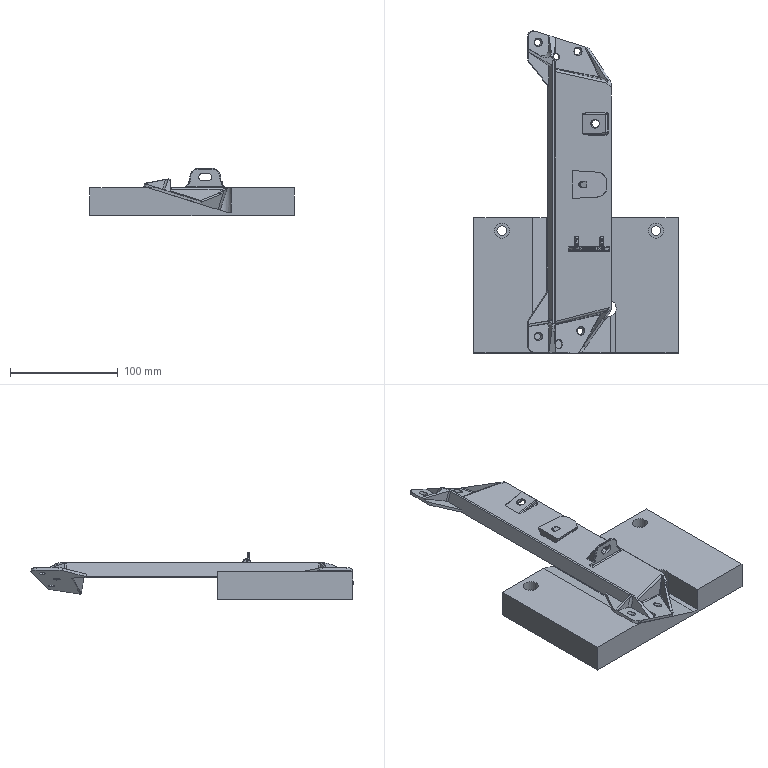NC program | NX | posted with a generic post | part box 190 x 299.709 x 43.804 mm
Lines 1 to 1011 of 6802:
N10 G17 G21 G94 G90
(G-型腔铣-粗 , TOOL : D6-粗刀)
N12 T01 M6
N14 G53
N16 G17 G0 G90 X-26.385 Y-5.888 S5300 M3
N18 G43 Z10. H1
N20 Z0.7
N22 G94 G1 Z-0.3 F2300.
N24 G2 X-29.15 Y-1.613 R3.6
N26 G3 X-28.979 Y0.112 R7.702
N28 G1 Y13.311
N30 G2 X-28.818 Y13.677 R0.5
N32 G3 X-28.659 Y14.001 R0.5
N34 G1 X-28.331 Y17.785
N36 G3 X-28.679 Y18.305 R0.5
N38 G1 X-32.101 Y19.378
N40 X-32.247 Y19.401
N42 X-32.98
N44 G3 X-33.479 Y18.902 R0.5
N46 G1 Y0.073
N48 G2 X-33.737 Y-1.258 R3.202
N50 X-35.553 Y-2.995 R3.2
N52 G3 X-37.656 Y-7.632 R3.6
N54 G1 Z0.7
N56 G0 Z3.
N58 X-26.385 Y-5.888
N60 Z0.401
N62 G1 Z-0.599
N64 G2 X-29.15 Y-1.613 R3.6
N66 G3 X-28.979 Y0.112 R7.702
N68 G1 Y13.311
N70 G2 X-28.818 Y13.677 R0.5
N72 G3 X-28.659 Y14.001 R0.5
N74 G1 X-28.331 Y17.785
N76 G3 X-28.679 Y18.305 R0.5
N78 G1 X-32.101 Y19.378
N80 X-32.247 Y19.401
N82 X-32.98
N84 G3 X-33.479 Y18.902 R0.5
N86 G1 Y0.073
N88 G2 X-33.737 Y-1.258 R3.202
N90 X-35.553 Y-2.995 R3.2
N92 G3 X-37.656 Y-7.632 R3.6
N94 G1 Z0.401
N96 G0 Z3.
N98 X-26.385 Y-5.888
N100 Z0.101
N102 G1 Z-0.899
N104 G2 X-29.15 Y-1.613 R3.6
N106 G3 X-28.979 Y0.112 R7.702
N108 G1 Y13.311
N110 G2 X-28.818 Y13.677 R0.5
N112 G3 X-28.659 Y14.001 R0.5
N114 G1 X-28.331 Y17.785
N116 G3 X-28.679 Y18.305 R0.5
N118 G1 X-32.101 Y19.378
N120 X-32.247 Y19.401
N122 X-32.98
N124 G3 X-33.479 Y18.902 R0.5
N126 G1 Y0.073
N128 G2 X-33.737 Y-1.258 R3.202
N130 X-35.553 Y-2.995 R3.2
N132 G3 X-37.656 Y-7.632 R3.6
N134 G1 Z0.101
N136 G0 Z3.
N138 X-26.385 Y-5.888
N140 Z-0.199
N142 G1 Z-1.199
N144 G2 X-29.15 Y-1.613 R3.6
N146 G3 X-28.979 Y0.112 R7.702
N148 G1 Y13.311
N150 G2 X-28.818 Y13.677 R0.5
N152 G3 X-28.659 Y14.001 R0.5
N154 G1 X-28.331 Y17.785
N156 G3 X-28.679 Y18.305 R0.5
N158 G1 X-32.101 Y19.378
N160 X-32.247 Y19.401
N162 X-32.98
N164 G3 X-33.479 Y18.902 R0.5
N166 G1 Y0.073
N168 G2 X-33.737 Y-1.258 R3.202
N170 X-35.553 Y-2.995 R3.2
N172 G3 X-37.656 Y-7.632 R3.6
N174 G1 Z-0.199
N176 G0 Z3.
N178 X-26.385 Y-5.888
N180 Z-0.498
N182 G1 Z-1.498
N184 G2 X-29.15 Y-1.613 R3.6
N186 G3 X-28.979 Y0.112 R7.702
N188 G1 Y13.312
N190 G2 X-28.818 Y13.677 R0.5
N192 G3 X-28.659 Y14.001 R0.5
N194 G1 X-28.331 Y17.785
N196 G3 X-28.679 Y18.305 R0.5
N198 G1 X-32.102 Y19.378
N200 X-32.246 Y19.401
N202 X-32.98
N204 G3 X-33.479 Y18.902 R0.5
N206 G1 Y0.073
N208 G2 X-33.737 Y-1.258 R3.202
N210 X-35.553 Y-2.995 R3.2
N212 G3 X-37.656 Y-7.632 R3.6
N214 G1 Z-0.498
N216 G0 Z3.
N218 X-26.385 Y-5.888
N220 Z-0.798
N222 G1 Z-1.798
N224 G2 X-29.15 Y-1.613 R3.6
N226 G3 X-28.979 Y0.112 R7.702
N228 G1 Y13.312
N230 G2 X-28.818 Y13.677 R0.5
N232 G3 X-28.659 Y14.001 R0.5
N234 G1 X-28.331 Y17.785
N236 G3 X-28.679 Y18.305 R0.5
N238 G1 X-32.102 Y19.378
N240 X-32.246 Y19.401
N242 X-32.98
N244 G3 X-33.479 Y18.902 R0.5
N246 G1 Y0.073
N248 G2 X-33.737 Y-1.257 R3.202
N250 X-35.553 Y-2.995 R3.2
N252 G3 X-37.656 Y-7.632 R3.6
N254 G1 Z-0.798
N256 G0 Z3.
N258 X-26.385 Y-5.888
N260 Z-1.098
N262 G1 Z-2.098
N264 G2 X-29.15 Y-1.613 R3.6
N266 G3 X-28.979 Y0.112 R7.702
N268 G1 Y13.312
N270 G2 X-28.818 Y13.677 R0.5
N272 G3 X-28.659 Y14.001 R0.5
N274 G1 X-28.331 Y17.785
N276 G3 X-28.679 Y18.305 R0.5
N278 G1 X-32.102 Y19.379
N280 X-32.246 Y19.401
N282 X-32.98
N284 G3 X-33.479 Y18.902 R0.5
N286 G1 Y0.073
N288 G2 X-33.736 Y-1.257 R3.202
N290 X-35.553 Y-2.995 R3.2
N292 G3 X-37.656 Y-7.632 R3.6
N294 G1 Z-1.098
N296 G0 Z3.
N298 X-26.385 Y-5.888
N300 Z-1.397
N302 G1 Z-2.397
N304 G2 X-29.15 Y-1.613 R3.6
N306 G3 X-28.979 Y0.112 R7.702
N308 G1 Y13.312
N310 G2 X-28.818 Y13.677 R0.5
N312 G3 X-28.659 Y14.001 R0.5
N314 G1 X-28.331 Y17.785
N316 G3 X-28.679 Y18.305 R0.5
N318 G1 X-32.102 Y19.379
N320 X-32.246 Y19.401
N322 X-32.98
N324 G3 X-33.479 Y18.902 R0.5
N326 G1 Y0.073
N328 G2 X-33.736 Y-1.257 R3.202
N330 X-35.553 Y-2.995 R3.2
N332 G3 X-37.656 Y-7.632 R3.6
N334 G1 Z-1.397
N336 G0 Z3.
N338 X-26.385 Y-5.888
N340 Z-1.697
N342 G1 Z-2.697
N344 G2 X-29.15 Y-1.613 R3.6
N346 G3 X-28.979 Y0.112 R7.702
N348 G1 Y13.312
N350 G2 X-28.818 Y13.677 R0.5
N352 G3 X-28.659 Y14.001 R0.5
N354 G1 X-28.331 Y17.785
N356 G3 X-28.679 Y18.305 R0.5
N358 G1 X-32.102 Y19.379
N360 X-32.246 Y19.401
N362 X-32.98
N364 G3 X-33.479 Y18.902 R0.5
N366 G1 Y0.073
N368 G2 X-33.736 Y-1.257 R3.202
N370 X-35.553 Y-2.995 R3.2
N372 G3 X-37.656 Y-7.632 R3.6
N374 G1 Z-1.697
N376 G0 Z3.
N378 X-26.385 Y-5.888
N380 Z-1.997
N382 G1 Z-2.997
N384 G2 X-29.15 Y-1.613 R3.6
N386 G3 X-28.979 Y0.112 R7.702
N388 G1 Y13.312
N390 G2 X-28.818 Y13.677 R0.5
N392 G3 X-28.659 Y14.001 R0.5
N394 G1 X-28.331 Y17.785
N396 G3 X-28.679 Y18.305 R0.5
N398 G1 X-32.102 Y19.379
N400 X-32.246 Y19.401
N402 X-32.98
N404 G3 X-33.479 Y18.902 R0.5
N406 G1 Y0.073
N408 G2 X-33.736 Y-1.257 R3.202
N410 X-35.553 Y-2.995 R3.2
N412 G3 X-37.656 Y-7.632 R3.6
N414 G1 Z-1.997
N416 G0 Z3.
N418 X-26.385 Y-5.888
N420 Z-2.296
N422 G1 Z-3.296
N424 G2 X-29.15 Y-1.613 R3.6
N426 G3 X-28.979 Y0.112 R7.702
N428 G1 Y13.313
N430 G2 X-28.818 Y13.677 R0.5
N432 G3 X-28.659 Y14.001 R0.5
N434 G1 X-28.331 Y17.785
N436 G3 X-28.679 Y18.305 R0.5
N438 G1 X-32.102 Y19.379
N440 X-32.246 Y19.401
N442 X-32.98
N444 G3 X-33.479 Y18.902 R0.5
N446 G1 Y0.073
N448 G2 X-33.736 Y-1.257 R3.202
N450 X-35.553 Y-2.995 R3.2
N452 G3 X-37.656 Y-7.632 R3.6
N454 G1 Z-2.296
N456 G0 Z3.
N458 X-26.385 Y-5.888
N460 Z-2.596
N462 G1 Z-3.596
N464 G2 X-29.15 Y-1.613 R3.6
N466 G3 X-28.979 Y0.112 R7.702
N468 G1 Y13.313
N470 G2 X-28.818 Y13.677 R0.5
N472 G3 X-28.659 Y14.001 R0.5
N474 G1 X-28.331 Y17.785
N476 G3 X-28.679 Y18.305 R0.5
N478 G1 X-32.103 Y19.379
N480 X-32.245 Y19.401
N482 X-32.98
N484 G3 X-33.479 Y18.902 R0.5
N486 G1 Y0.073
N488 G2 X-33.736 Y-1.257 R3.202
N490 X-35.553 Y-2.995 R3.2
N492 G3 X-37.656 Y-7.632 R3.6
N494 G1 Z-2.596
N496 G0 Z3.
N498 X-26.385 Y-5.888
N500 Z-2.896
N502 G1 Z-3.896
N504 G2 X-29.15 Y-1.613 R3.6
N506 G3 X-28.979 Y0.112 R7.702
N508 G1 Y13.313
N510 G2 X-28.818 Y13.677 R0.5
N512 G3 X-28.659 Y14.001 R0.5
N514 G1 X-28.331 Y17.785
N516 G3 X-28.679 Y18.305 R0.5
N518 G1 X-32.103 Y19.379
N520 X-32.245 Y19.401
N522 X-32.98
N524 G3 X-33.479 Y18.902 R0.5
N526 G1 Y0.073
N528 G2 X-33.736 Y-1.257 R3.202
N530 X-35.553 Y-2.995 R3.2
N532 G3 X-37.656 Y-7.632 R3.6
N534 G1 Z-2.896
N536 G0 Z3.
N538 X-26.385 Y-5.888
N540 Z-3.195
N542 G1 Z-4.195
N544 G2 X-29.15 Y-1.613 R3.6
N546 G3 X-28.979 Y0.112 R7.702
N548 G1 Y13.313
N550 G2 X-28.818 Y13.677 R0.5
N552 G3 X-28.659 Y14.001 R0.5
N554 G1 X-28.331 Y17.785
N556 G3 X-28.679 Y18.305 R0.5
N558 G1 X-32.103 Y19.379
N560 X-32.245 Y19.401
N562 X-32.98
N564 G3 X-33.479 Y18.902 R0.5
N566 G1 Y0.073
N568 G2 X-33.736 Y-1.256 R3.202
N570 X-35.553 Y-2.995 R3.2
N572 G3 X-37.656 Y-7.632 R3.6
N574 G1 Z-3.195
N576 G0 Z3.
N578 X-26.385 Y-5.888
N580 Z-3.495
N582 G1 Z-4.495
N584 G2 X-29.15 Y-1.613 R3.6
N586 G3 X-28.979 Y0.112 R7.702
N588 G1 Y13.313
N590 G2 X-28.818 Y13.677 R0.5
N592 G3 X-28.659 Y14.001 R0.5
N594 G1 X-28.331 Y17.785
N596 G3 X-28.679 Y18.305 R0.5
N598 G1 X-32.103 Y19.379
N600 X-32.245 Y19.401
N602 X-32.98
N604 G3 X-33.479 Y18.902 R0.5
N606 G1 Y0.073
N608 G2 X-33.736 Y-1.256 R3.202
N610 X-35.553 Y-2.995 R3.2
N612 G3 X-37.656 Y-7.632 R3.6
N614 G1 Z-3.495
N616 G0 Z3.
N618 X-26.385 Y-5.888
N620 Z-3.795
N622 G1 Z-4.795
N624 G2 X-29.15 Y-1.613 R3.6
N626 G3 X-28.979 Y0.112 R7.702
N628 G1 Y13.313
N630 G2 X-28.818 Y13.677 R0.5
N632 G3 X-28.659 Y14.001 R0.5
N634 G1 X-28.331 Y17.785
N636 G3 X-28.679 Y18.305 R0.5
N638 G1 X-32.103 Y19.379
N640 X-32.245 Y19.401
N642 X-32.98
N644 G3 X-33.479 Y18.902 R0.5
N646 G1 Y0.073
N648 G2 X-33.736 Y-1.256 R3.202
N650 X-35.553 Y-2.995 R3.2
N652 G3 X-37.656 Y-7.632 R3.6
N654 G1 Z-3.795
N656 G0 Z3.
N658 X-26.385 Y-5.888
N660 Z-4.094
N662 G1 Z-5.094
N664 G2 X-29.15 Y-1.613 R3.6
N666 G3 X-28.979 Y0.112 R7.702
N668 G1 Y13.313
N670 G2 X-28.818 Y13.677 R0.5
N672 G3 X-28.659 Y14.001 R0.5
N674 G1 X-28.331 Y17.785
N676 G3 X-28.679 Y18.305 R0.5
N678 G1 X-32.103 Y19.379
N680 X-32.245 Y19.401
N682 X-32.98
N684 G3 X-33.479 Y18.902 R0.5
N686 G1 Y0.073
N688 G2 X-33.736 Y-1.256 R3.202
N690 X-35.553 Y-2.995 R3.2
N692 G3 X-37.656 Y-7.632 R3.6
N694 G1 Z-4.094
N696 G0 Z3.
N698 X-26.385 Y-5.888
N700 Z-4.394
N702 G1 Z-5.394
N704 G2 X-29.15 Y-1.613 R3.6
N706 G3 X-28.979 Y0.112 R7.702
N708 G1 Y13.313
N710 G2 X-28.818 Y13.677 R0.5
N712 G3 X-28.659 Y14.001 R0.5
N714 G1 X-28.331 Y17.785
N716 G3 X-28.679 Y18.305 R0.5
N718 G1 X-32.103 Y19.379
N720 X-32.245 Y19.401
N722 X-32.981
N724 G3 X-33.479 Y18.902 R0.5
N726 G1 Y0.073
N728 G2 X-33.736 Y-1.256 R3.202
N730 X-35.553 Y-2.995 R3.2
N732 G3 X-37.656 Y-7.632 R3.6
N734 G1 Z-4.394
N736 G0 Z3.
N738 X-26.385 Y-5.888
N740 Z-4.694
N742 G1 Z-5.694
N744 G2 X-29.15 Y-1.613 R3.6
N746 G3 X-28.979 Y0.112 R7.702
N748 G1 Y13.314
N750 G2 X-28.818 Y13.677 R0.5
N752 G3 X-28.659 Y14.001 R0.5
N754 G1 X-28.331 Y17.785
N756 G3 X-28.679 Y18.305 R0.5
N758 G1 X-32.103 Y19.379
N760 X-32.245 Y19.401
N762 X-32.981
N764 G3 X-33.479 Y18.902 R0.5
N766 G1 Y0.073
N768 G2 X-33.736 Y-1.256 R3.202
N770 X-35.553 Y-2.995 R3.2
N772 G3 X-37.656 Y-7.632 R3.6
N774 G1 Z-4.694
N776 G0 Z3.
N778 X-26.385 Y-5.888
N780 Z-4.993
N782 G1 Z-5.993
N784 G2 X-29.15 Y-1.613 R3.6
N786 G3 X-28.979 Y0.112 R7.702
N788 G1 Y13.314
N790 G2 X-28.818 Y13.677 R0.5
N792 G3 X-28.659 Y14.001 R0.5
N794 G1 X-28.331 Y17.785
N796 G3 X-28.679 Y18.305 R0.5
N798 G1 X-32.103 Y19.379
N800 X-32.244 Y19.401
N802 X-32.981
N804 G3 X-33.479 Y18.902 R0.5
N806 G1 Y0.073
N808 G2 X-33.736 Y-1.256 R3.202
N810 X-35.553 Y-2.995 R3.2
N812 G3 X-37.656 Y-7.632 R3.6
N814 G1 Z-4.993
N816 G0 Z3.
N818 X-26.385 Y-5.888
N820 Z-5.293
N822 G1 Z-6.293
N824 G2 X-29.15 Y-1.613 R3.6
N826 G3 X-28.979 Y0.112 R7.702
N828 G1 Y13.314
N830 G2 X-28.818 Y13.677 R0.5
N832 G3 X-28.659 Y14.001 R0.5
N834 G1 X-28.331 Y17.785
N836 G3 X-28.679 Y18.305 R0.5
N838 G1 X-32.104 Y19.379
N840 X-32.244 Y19.401
N842 X-32.981
N844 G3 X-33.479 Y18.902 R0.5
N846 G1 Y0.073
N848 G2 X-33.736 Y-1.256 R3.202
N850 X-35.553 Y-2.995 R3.2
N852 G3 X-37.656 Y-7.632 R3.6
N854 G1 Z-5.293
N856 G0 Z3.
N858 X-26.385 Y-5.888
N860 Z-5.593
N862 G1 Z-6.593
N864 G2 X-29.15 Y-1.613 R3.6
N866 G3 X-28.979 Y0.112 R7.702
N868 G1 Y13.314
N870 G2 X-28.818 Y13.677 R0.5
N872 G3 X-28.659 Y14.001 R0.5
N874 G1 X-28.331 Y17.785
N876 G3 X-28.679 Y18.305 R0.5
N878 G1 X-32.104 Y19.379
N880 X-32.244 Y19.401
N882 X-32.981
N884 G3 X-33.479 Y18.902 R0.5
N886 G1 Y0.073
N888 G2 X-33.736 Y-1.256 R3.202
N890 X-35.553 Y-2.995 R3.2
N892 G3 X-37.656 Y-7.632 R3.6
N894 G1 Z-5.593
N896 G0 Z3.
N898 X-26.385 Y-5.888
N900 Z-5.892
N902 G1 Z-6.892
N904 G2 X-29.15 Y-1.613 R3.6
N906 G3 X-28.979 Y0.112 R7.702
N908 G1 Y13.314
N910 G2 X-28.818 Y13.677 R0.5
N912 G3 X-28.659 Y14.001 R0.5
N914 G1 X-28.331 Y17.785
N916 G3 X-28.679 Y18.305 R0.5
N918 G1 X-32.104 Y19.379
N920 X-32.244 Y19.401
N922 X-32.981
N924 G3 X-33.479 Y18.902 R0.5
N926 G1 Y0.073
N928 G2 X-33.736 Y-1.256 R3.202
N930 X-35.553 Y-2.995 R3.2
N932 G3 X-37.656 Y-7.632 R3.6
N934 G1 Z-5.892
N936 G0 Z3.
N938 X-26.385 Y-5.888
N940 Z-6.192
N942 G1 Z-7.192
N944 G2 X-29.15 Y-1.613 R3.6
N946 G3 X-28.979 Y0.112 R7.702
N948 G1 Y13.314
N950 G2 X-28.818 Y13.677 R0.5
N952 G3 X-28.659 Y14.001 R0.5
N954 G1 X-28.331 Y17.785
N956 G3 X-28.679 Y18.305 R0.5
N958 G1 X-32.104 Y19.379
N960 X-32.244 Y19.401
N962 X-32.981
N964 G3 X-33.479 Y18.902 R0.5
N966 G1 Y0.073
N968 G2 X-33.736 Y-1.255 R3.202
N970 X-35.553 Y-2.995 R3.2
N972 G3 X-37.656 Y-7.632 R3.6
N974 G1 Z-6.192
N976 G0 Z3.
N978 X-26.385 Y-5.888
N980 Z-6.492
N982 G1 Z-7.492
N984 G2 X-29.15 Y-1.613 R3.6
N986 G3 X-28.979 Y0.112 R7.702
N988 G1 Y13.314
N990 G2 X-28.818 Y13.677 R0.5
N992 G3 X-28.659 Y14.001 R0.5
N994 G1 X-28.331 Y17.785
N996 G3 X-28.679 Y18.305 R0.5
N998 G1 X-32.104 Y19.379
N1000 X-32.244 Y19.401
N1002 X-32.981
N1004 G3 X-33.479 Y18.902 R0.5
N1006 G1 Y0.073
N1008 G2 X-33.736 Y-1.255 R3.202
N1010 X-35.553 Y-2.995 R3.2
N1012 G3 X-37.656 Y-7.632 R3.6
N1014 G1 Z-6.492
N1016 G0 Z3.
N1018 X-26.385 Y-5.888
N1020 Z-6.791
N1022 G1 Z-7.791
N1024 G2 X-29.15 Y-1.613 R3.6
N1026 G3 X-28.979 Y0.112 R7.702
N1028 G1 Y13.314
N1030 G2 X-28.818 Y13.677 R0.5
N1032 G3 X-28.659 Y14.001 R0.5
N1034 G1 X-28.331 Y17.785
N1036 G3 X-28.679 Y18.305 R0.5
N1038 G1 X-32.104 Y19.379
N1040 X-32.244 Y19.401
N1042 X-32.981
N1044 G3 X-33.479 Y18.902 R0.5
N1046 G1 Y0.073
N1048 G2 X-33.735 Y-1.255 R3.202
N1050 X-35.553 Y-2.995 R3.2
N1052 G3 X-37.656 Y-7.632 R3.6
N1054 G1 Z-6.791
N1056 G0 Z3.
N1058 X-26.385 Y-5.888
N1060 Z-7.091
N1062 G1 Z-8.091
N1064 G2 X-29.15 Y-1.613 R3.6
N1066 G3 X-28.979 Y0.112 R7.702
N1068 G1 Y13.314
N1070 G2 X-28.818 Y13.677 R0.5
N1072 G3 X-28.659 Y14.001 R0.5
N1074 G1 X-28.331 Y17.785
N1076 G3 X-28.679 Y18.305 R0.5
N1078 G1 X-32.104 Y19.379
N1080 X-32.244 Y19.401
N1082 X-32.981
N1084 G3 X-33.479 Y18.902 R0.5
N1086 G1 Y0.073
N1088 G2 X-33.735 Y-1.255 R3.202
N1090 X-35.553 Y-2.995 R3.2
N1092 G3 X-37.656 Y-7.632 R3.6
N1094 G1 Z-7.091
N1096 G0 Z3.
N1098 X-26.385 Y-5.888
N1100 Z-7.391
N1102 G1 Z-8.391
N1104 G2 X-29.15 Y-1.613 R3.6
N1106 G3 X-28.979 Y0.112 R7.702
N1108 G1 Y13.314
N1110 G2 X-28.818 Y13.677 R0.5
N1112 G3 X-28.659 Y14.001 R0.5
N1114 G1 X-28.331 Y17.785
N1116 G3 X-28.679 Y18.305 R0.5
N1118 G1 X-32.104 Y19.379
N1120 X-32.244 Y19.401
N1122 X-32.981
N1124 G3 X-33.479 Y18.902 R0.5
N1126 G1 Y0.073
N1128 G2 X-33.735 Y-1.255 R3.202
N1130 X-35.553 Y-2.995 R3.2
N1132 G3 X-37.656 Y-7.632 R3.6
N1134 G1 Z-7.391
N1136 G0 Z3.
N1138 X-26.385 Y-5.888
N1140 Z-7.69
N1142 G1 Z-8.69
N1144 G2 X-29.15 Y-1.613 R3.6
N1146 G3 X-28.979 Y0.112 R7.702
N1148 G1 Y13.315
N1150 G2 X-28.818 Y13.677 R0.5
N1152 G3 X-28.659 Y14.001 R0.5
N1154 G1 X-28.331 Y17.785
N1156 G3 X-28.679 Y18.305 R0.5
N1158 G1 X-32.104 Y19.379
N1160 X-32.244 Y19.401
N1162 X-32.981
N1164 G3 X-33.479 Y18.902 R0.5
N1166 G1 Y0.073
N1168 G2 X-33.735 Y-1.255 R3.202
N1170 X-35.553 Y-2.995 R3.2
N1172 G3 X-37.656 Y-7.632 R3.6
N1174 G1 Z-7.69
N1176 G0 Z3.
N1178 X-26.385 Y-5.888
N1180 Z-7.99
N1182 G1 Z-8.99
N1184 G2 X-29.15 Y-1.613 R3.6
N1186 G3 X-28.979 Y0.112 R7.702
N1188 G1 Y13.315
N1190 G2 X-28.818 Y13.677 R0.5
N1192 G3 X-28.659 Y14.001 R0.5
N1194 G1 X-28.331 Y17.785
N1196 G3 X-28.679 Y18.305 R0.5
N1198 G1 X-32.104 Y19.379
N1200 X-32.243 Y19.401
N1202 X-32.981
N1204 G3 X-33.479 Y18.902 R0.5
N1206 G1 Y0.073
N1208 G2 X-33.735 Y-1.254 R3.202
N1210 X-35.553 Y-2.995 R3.2
N1212 G3 X-37.656 Y-7.632 R3.6
N1214 G1 Z-7.99
N1216 G0 Z3.
N1218 X-26.385 Y-5.888
N1220 Z-8.29
N1222 G1 Z-9.29
N1224 G2 X-29.15 Y-1.613 R3.6
N1226 G3 X-28.979 Y0.112 R7.702
N1228 G1 Y13.315
N1230 G2 X-28.818 Y13.677 R0.5
N1232 G3 X-28.659 Y14.001 R0.5
N1234 G1 X-28.331 Y17.785
N1236 G3 X-28.679 Y18.305 R0.5
N1238 G1 X-32.104 Y19.379
N1240 X-32.243 Y19.401
N1242 X-32.981
N1244 G3 X-33.479 Y18.902 R0.5
N1246 G1 Y0.073
N1248 G2 X-33.735 Y-1.254 R3.202
N1250 X-35.553 Y-2.995 R3.2
N1252 G3 X-37.656 Y-7.632 R3.6
N1254 G1 Z-8.29
N1256 G0 Z3.
N1258 X-26.385 Y-5.888
N1260 Z-8.589
N1262 G1 Z-9.589
N1264 G2 X-29.15 Y-1.613 R3.6
N1266 G3 X-28.979 Y0.112 R7.702
N1268 G1 Y13.315
N1270 G2 X-28.818 Y13.677 R0.5
N1272 G3 X-28.659 Y14.001 R0.5
N1274 G1 X-28.331 Y17.785
N1276 G3 X-28.679 Y18.305 R0.5
N1278 G1 X-32.105 Y19.379
N1280 X-32.243 Y19.401
N1282 X-32.981
N1284 G3 X-33.479 Y18.902 R0.5
N1286 G1 Y0.073
N1288 G2 X-33.735 Y-1.254 R3.202
N1290 X-35.553 Y-2.995 R3.2
N1292 G3 X-37.656 Y-7.632 R3.6
N1294 G1 Z-8.589
N1296 G0 Z3.
N1298 X-26.385 Y-5.888
N1300 Z-8.889
N1302 G1 Z-9.889
N1304 G2 X-29.15 Y-1.613 R3.6
N1306 G3 X-28.979 Y0.112 R7.702
N1308 G1 Y13.315
N1310 G2 X-28.818 Y13.677 R0.5
N1312 G3 X-28.659 Y14.001 R0.5
N1314 G1 X-28.331 Y17.785
N1316 G3 X-28.679 Y18.305 R0.5
N1318 G1 X-32.105 Y19.379
N1320 X-32.243 Y19.401
N1322 X-32.981
N1324 G3 X-33.479 Y18.902 R0.5
N1326 G1 Y0.073
N1328 G2 X-33.735 Y-1.254 R3.202
N1330 X-35.553 Y-2.995 R3.2
N1332 G3 X-37.656 Y-7.632 R3.6
N1334 G1 Z-8.889
N1336 G0 Z3.
N1338 X-26.385 Y-5.888
N1340 Z-9.189
N1342 G1 Z-10.189
N1344 G2 X-29.15 Y-1.613 R3.6
N1346 G3 X-28.979 Y0.112 R7.702
N1348 G1 Y13.315
N1350 G2 X-28.818 Y13.677 R0.5
N1352 G3 X-28.659 Y14.001 R0.5
N1354 G1 X-28.331 Y17.785
N1356 G3 X-28.679 Y18.305 R0.5
N1358 G1 X-32.105 Y19.379
N1360 X-32.243 Y19.401
N1362 X-32.981
N1364 G3 X-33.479 Y18.902 R0.5
N1366 G1 Y0.073
N1368 G2 X-33.735 Y-1.254 R3.202
N1370 X-35.553 Y-2.995 R3.2
N1372 G3 X-37.656 Y-7.632 R3.6
N1374 G1 Z-9.189
N1376 G0 Z3.
N1378 X-26.385 Y-5.888
N1380 Z-9.488
N1382 G1 Z-10.488
N1384 G2 X-29.15 Y-1.613 R3.6
N1386 G3 X-28.979 Y0.112 R7.702
N1388 G1 Y13.315
N1390 G2 X-28.818 Y13.677 R0.5
N1392 G3 X-28.659 Y14.001 R0.5
N1394 G1 X-28.331 Y17.785
N1396 G3 X-28.679 Y18.305 R0.5
N1398 G1 X-32.105 Y19.379
N1400 X-32.243 Y19.401
N1402 X-32.981
N1404 G3 X-33.479 Y18.902 R0.5
N1406 G1 Y0.073
N1408 G2 X-33.735 Y-1.254 R3.202
N1410 X-35.553 Y-2.995 R3.2
N1412 G3 X-37.656 Y-7.632 R3.6
N1414 G1 Z-9.488
N1416 G0 Z3.
N1418 X-26.385 Y-5.888
N1420 Z-9.788
N1422 G1 Z-10.788
N1424 G2 X-29.15 Y-1.613 R3.6
N1426 G3 X-28.979 Y0.112 R7.702
N1428 G1 Y13.315
N1430 G2 X-28.818 Y13.677 R0.5
N1432 G3 X-28.659 Y14.001 R0.5
N1434 G1 X-28.331 Y17.785
N1436 G3 X-28.679 Y18.305 R0.5
N1438 G1 X-32.105 Y19.379
N1440 X-32.243 Y19.401
N1442 X-32.981
N1444 G3 X-33.479 Y18.902 R0.5
N1446 G1 Y0.073
N1448 G2 X-33.735 Y-1.254 R3.202
N1450 X-35.553 Y-2.995 R3.2
N1452 G3 X-37.656 Y-7.632 R3.6
N1454 G1 Z-9.788
N1456 G0 Z3.
N1458 X-26.385 Y-5.888
N1460 Z-10.088
N1462 G1 Z-11.088
N1464 G2 X-29.15 Y-1.613 R3.6
N1466 G3 X-28.979 Y0.112 R7.702
N1468 G1 Y13.315
N1470 G2 X-28.818 Y13.677 R0.5
N1472 G3 X-28.659 Y14.001 R0.5
N1474 G1 X-28.331 Y17.785
N1476 G3 X-28.679 Y18.305 R0.5
N1478 G1 X-32.105 Y19.379
N1480 X-32.243 Y19.401
N1482 X-32.981
N1484 G3 X-33.479 Y18.902 R0.5
N1486 G1 Y0.073
N1488 G2 X-33.741 Y-1.269 R3.202
N1490 X-35.553 Y-2.995 R3.2
N1492 G3 X-37.656 Y-7.632 R3.6
N1494 G1 Z-10.088
N1496 G0 Z3.
N1498 X-26.385 Y-5.888
N1500 Z-10.387
N1502 G1 Z-11.387
N1504 G2 X-29.15 Y-1.613 R3.6
N1506 G3 X-28.979 Y0.112 R7.702
N1508 G1 Y13.315
N1510 G2 X-28.818 Y13.677 R0.5
N1512 G3 X-28.659 Y14.001 R0.5
N1514 G1 X-28.331 Y17.785
N1516 G3 X-28.679 Y18.305 R0.5
N1518 G1 X-32.105 Y19.38
N1520 X-32.243 Y19.401
N1522 X-32.981
N1524 G3 X-33.479 Y18.902 R0.5
N1526 G1 Y0.073
N1528 G2 X-33.735 Y-1.254 R3.202
N1530 X-35.553 Y-2.995 R3.2
N1532 G3 X-37.656 Y-7.632 R3.6
N1534 G1 Z-10.387
N1536 G0 Z3.
N1538 X-26.385 Y-5.888
N1540 Z-10.687
N1542 G1 Z-11.687
N1544 G2 X-29.15 Y-1.613 R3.6
N1546 G3 X-28.979 Y0.112 R7.702
N1548 G1 Y13.315
N1550 G2 X-28.818 Y13.677 R0.5
N1552 G3 X-28.659 Y14.001 R0.5
N1554 G1 X-28.331 Y17.785
N1556 G3 X-28.679 Y18.305 R0.5
N1558 G1 X-32.105 Y19.38
N1560 X-32.243 Y19.401
N1562 X-32.981
N1564 G3 X-33.479 Y18.902 R0.5
N1566 G1 Y0.073
N1568 G2 X-33.735 Y-1.254 R3.202
N1570 X-35.553 Y-2.995 R3.2
N1572 G3 X-37.656 Y-7.632 R3.6
N1574 G1 Z-10.687
N1576 G0 Z3.
N1578 X-26.385 Y-5.888
N1580 Z-10.987
N1582 G1 Z-11.987
N1584 G2 X-29.15 Y-1.613 R3.6
N1586 G3 X-28.979 Y0.112 R7.702
N1588 G1 Y13.315
N1590 G2 X-28.818 Y13.677 R0.5
N1592 G3 X-28.659 Y14.001 R0.5
N1594 G1 X-28.331 Y17.785
N1596 G3 X-28.679 Y18.305 R0.5
N1598 G1 X-32.105 Y19.38
N1600 X-32.243 Y19.401
N1602 X-32.981
N1604 G3 X-33.479 Y18.902 R0.5
N1606 G1 Y0.073
N1608 G2 X-33.735 Y-1.253 R3.202
N1610 X-35.553 Y-2.995 R3.2
N1612 G3 X-37.656 Y-7.632 R3.6
N1614 G1 Z-10.987
N1616 G0 Z3.
N1618 X-26.385 Y-5.888
N1620 Z-11.286
N1622 G1 Z-12.286
N1624 G2 X-29.15 Y-1.613 R3.6
N1626 G3 X-28.979 Y0.112 R7.702
N1628 G1 Y13.316
N1630 G2 X-28.818 Y13.677 R0.5
N1632 G3 X-28.659 Y14.001 R0.5
N1634 G1 X-28.331 Y17.785
N1636 G3 X-28.679 Y18.305 R0.5
N1638 G1 X-32.105 Y19.38
N1640 X-32.243 Y19.401
N1642 X-32.981
N1644 G3 X-33.479 Y18.902 R0.5
N1646 G1 Y0.073
N1648 G2 X-33.735 Y-1.253 R3.202
N1650 X-35.553 Y-2.995 R3.2
N1652 G3 X-37.656 Y-7.632 R3.6
N1654 G1 Z-11.286
N1656 G0 Z3.
N1658 X-26.385 Y-5.888
N1660 Z-11.586
N1662 G1 Z-12.586
N1664 G2 X-29.15 Y-1.613 R3.6
N1666 G3 X-28.979 Y0.112 R7.702
N1668 G1 Y13.316
N1670 G2 X-28.818 Y13.677 R0.5
N1672 G3 X-28.659 Y14.001 R0.5
N1674 G1 X-28.331 Y17.785
N1676 G3 X-28.679 Y18.305 R0.5
N1678 G1 X-32.105 Y19.38
N1680 X-32.243 Y19.401
N1682 X-32.981
N1684 G3 X-33.479 Y18.902 R0.5
N1686 G1 Y0.073
N1688 G2 X-33.735 Y-1.253 R3.202
N1690 X-35.553 Y-2.995 R3.2
N1692 G3 X-37.656 Y-7.632 R3.6
N1694 G1 Z-11.586
N1696 G0 Z3.
N1698 X-26.385 Y-5.888
N1700 Z-11.886
N1702 G1 Z-12.886
N1704 G2 X-29.15 Y-1.613 R3.6
N1706 G3 X-28.979 Y0.112 R7.702
N1708 G1 Y13.316
N1710 G2 X-28.818 Y13.677 R0.5
N1712 G3 X-28.659 Y14.001 R0.5
N1714 G1 X-28.331 Y17.785
N1716 G3 X-28.679 Y18.305 R0.5
N1718 G1 X-32.105 Y19.38
N1720 X-32.242 Y19.401
N1722 X-32.981
N1724 G3 X-33.479 Y18.902 R0.5
N1726 G1 Y0.073
N1728 G2 X-33.735 Y-1.253 R3.202
N1730 X-35.553 Y-2.995 R3.2
N1732 G3 X-37.656 Y-7.632 R3.6
N1734 G1 Z-11.886
N1736 G0 Z3.
N1738 X-26.385 Y-5.888
N1740 Z-12.185
N1742 G1 Z-13.185
N1744 G2 X-29.15 Y-1.613 R3.6
N1746 G3 X-28.979 Y0.112 R7.702
N1748 G1 Y13.316
N1750 G2 X-28.818 Y13.677 R0.5
N1752 G3 X-28.659 Y14.001 R0.5
N1754 G1 X-28.331 Y17.785
N1756 G3 X-28.679 Y18.305 R0.5
N1758 G1 X-32.105 Y19.38
N1760 X-32.242 Y19.401
N1762 X-32.981
N1764 G3 X-33.479 Y18.902 R0.5
N1766 G1 Y0.073
N1768 G2 X-33.735 Y-1.253 R3.202
N1770 X-35.553 Y-2.995 R3.2
N1772 G3 X-37.656 Y-7.632 R3.6
N1774 G1 Z-12.185
N1776 G0 Z3.
N1778 X-26.385 Y-5.888
N1780 Z-12.485
N1782 G1 Z-13.485
N1784 G2 X-29.15 Y-1.613 R3.6
N1786 G3 X-28.979 Y0.112 R7.702
N1788 G1 Y13.316
N1790 G2 X-28.818 Y13.677 R0.5
N1792 G3 X-28.659 Y14.001 R0.5
N1794 G1 X-28.331 Y17.785
N1796 G3 X-28.679 Y18.305 R0.5
N1798 G1 X-32.106 Y19.38
N1800 X-32.242 Y19.401
N1802 X-32.981
N1804 G3 X-33.479 Y18.902 R0.5
N1806 G1 Y0.073
N1808 G2 X-33.735 Y-1.253 R3.202
N1810 X-35.553 Y-2.995 R3.2
N1812 G3 X-37.656 Y-7.632 R3.6
N1814 G1 Z-12.485
N1816 G0 Z3.
N1818 X-26.385 Y-5.888
N1820 Z-12.785
N1822 G1 Z-13.785
N1824 G2 X-29.15 Y-1.613 R3.6
N1826 G3 X-28.979 Y0.112 R7.702
N1828 G1 Y13.316
N1830 G2 X-28.818 Y13.677 R0.5
N1832 G3 X-28.659 Y14.001 R0.5
N1834 G1 X-28.331 Y17.785
N1836 G3 X-28.679 Y18.305 R0.5
N1838 G1 X-32.106 Y19.38
N1840 X-32.242 Y19.401
N1842 X-32.981
N1844 G3 X-33.479 Y18.902 R0.5
N1846 G1 Y0.073
N1848 G2 X-33.734 Y-1.253 R3.202
N1850 X-35.553 Y-2.995 R3.2
N1852 G3 X-37.656 Y-7.632 R3.6
N1854 G1 Z-12.785
N1856 G0 Z3.
N1858 X-26.385 Y-5.888
N1860 Z-13.084
N1862 G1 Z-14.084
N1864 G2 X-29.15 Y-1.613 R3.6
N1866 G3 X-28.979 Y0.112 R7.702
N1868 G1 Y13.316
N1870 G2 X-28.818 Y13.677 R0.5
N1872 G3 X-28.659 Y14.001 R0.5
N1874 G1 X-28.331 Y17.785
N1876 G3 X-28.679 Y18.305 R0.5
N1878 G1 X-32.106 Y19.38
N1880 X-32.242 Y19.401
N1882 X-32.981
N1884 G3 X-33.479 Y18.902 R0.5
N1886 G1 Y0.073
N1888 G2 X-33.734 Y-1.253 R3.202
N1890 X-35.553 Y-2.995 R3.2
N1892 G3 X-37.656 Y-7.632 R3.6
N1894 G1 Z-13.084
N1896 G0 Z3.
N1898 X-26.385 Y-5.888
N1900 Z-13.384
N1902 G1 Z-14.384
N1904 G2 X-29.15 Y-1.613 R3.6
N1906 G3 X-28.979 Y0.112 R7.702
N1908 G1 Y13.316
N1910 G2 X-28.818 Y13.677 R0.5
N1912 G3 X-28.659 Y14.001 R0.5
N1914 G1 X-28.331 Y17.785
N1916 G3 X-28.679 Y18.305 R0.5
N1918 G1 X-32.106 Y19.38
N1920 X-32.242 Y19.401
N1922 X-32.981
N1924 G3 X-33.479 Y18.902 R0.5
N1926 G1 Y0.073
N1928 G2 X-33.734 Y-1.253 R3.202
N1930 X-35.553 Y-2.995 R3.2
N1932 G3 X-37.656 Y-7.632 R3.6
N1934 G1 Z-13.384
N1936 G0 Z3.
N1938 X-26.385 Y-5.888
N1940 Z-13.683
N1942 G1 Z-14.683
N1944 G2 X-29.15 Y-1.613 R3.6
N1946 G3 X-28.979 Y0.112 R7.702
N1948 G1 Y13.316
N1950 G2 X-28.818 Y13.677 R0.5
N1952 G3 X-28.659 Y14.001 R0.5
N1954 G1 X-28.331 Y17.785
N1956 G3 X-28.679 Y18.305 R0.5
N1958 G1 X-32.106 Y19.38
N1960 X-32.242 Y19.401
N1962 X-32.981
N1964 G3 X-33.479 Y18.902 R0.5
N1966 G1 Y0.073
N1968 G2 X-33.734 Y-1.253 R3.202
N1970 X-35.553 Y-2.995 R3.2
N1972 G3 X-37.656 Y-7.632 R3.6
N1974 G1 Z-13.683
N1976 G0 Z3.
N1978 X-26.385 Y-5.888
N1980 Z-13.983
N1982 G1 Z-14.983
N1984 G2 X-29.15 Y-1.613 R3.6
N1986 G3 X-28.979 Y0.112 R7.702
N1988 G1 Y13.316
N1990 G2 X-28.818 Y13.677 R0.5
N1992 G3 X-28.659 Y14.001 R0.5
N1994 G1 X-28.331 Y17.785
N1996 G3 X-28.679 Y18.305 R0.5
N1998 G1 X-32.106 Y19.38
N2000 X-32.242 Y19.401
N2002 X-32.981
N2004 G3 X-33.479 Y18.902 R0.5
N2006 G1 Y0.073
N2008 G2 X-33.734 Y-1.252 R3.202
N2010 X-35.553 Y-2.995 R3.2
N2012 G3 X-37.656 Y-7.632 R3.6
N2014 G1 Z-13.983
N2016 G0 Z3.
N2018 X-26.385 Y-5.888
N2020 Z-14.283